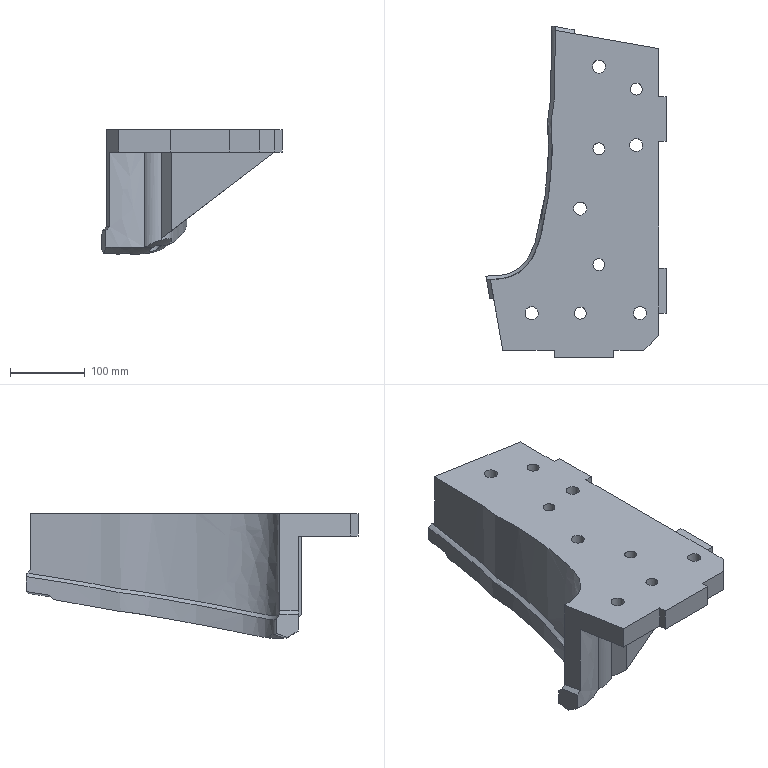Part | NX | features solid 2 | 1 solid | 72 faces | box 241.313 x 444.589 x 167.056 mm | volume 3536678 mm3 | plane 37 | cylinder 19 | spline 15 | cone 1 | commonest cylinder face diameters 16 x5 17.5 x5 25 x5 40 x2 14.5 x1 45 x1